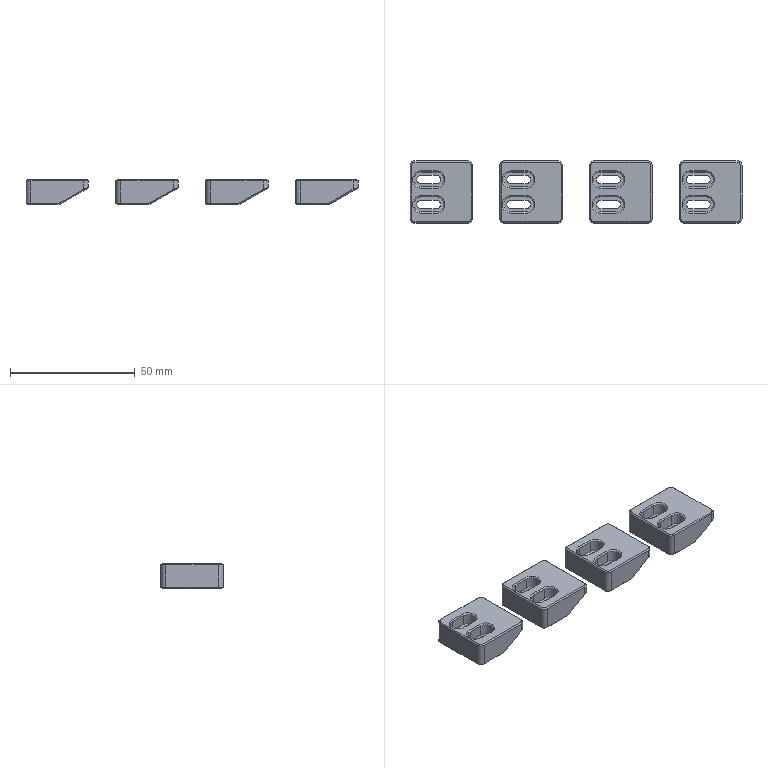Part | 4 solids | 232 faces | box 133 x 25 x 10 mm | volume 17190 mm3 | plane 124 | cylinder 52 | cone 48 | spline 8 | commonest cylinder face diameters 6 x20 3.5 x16 4 x16